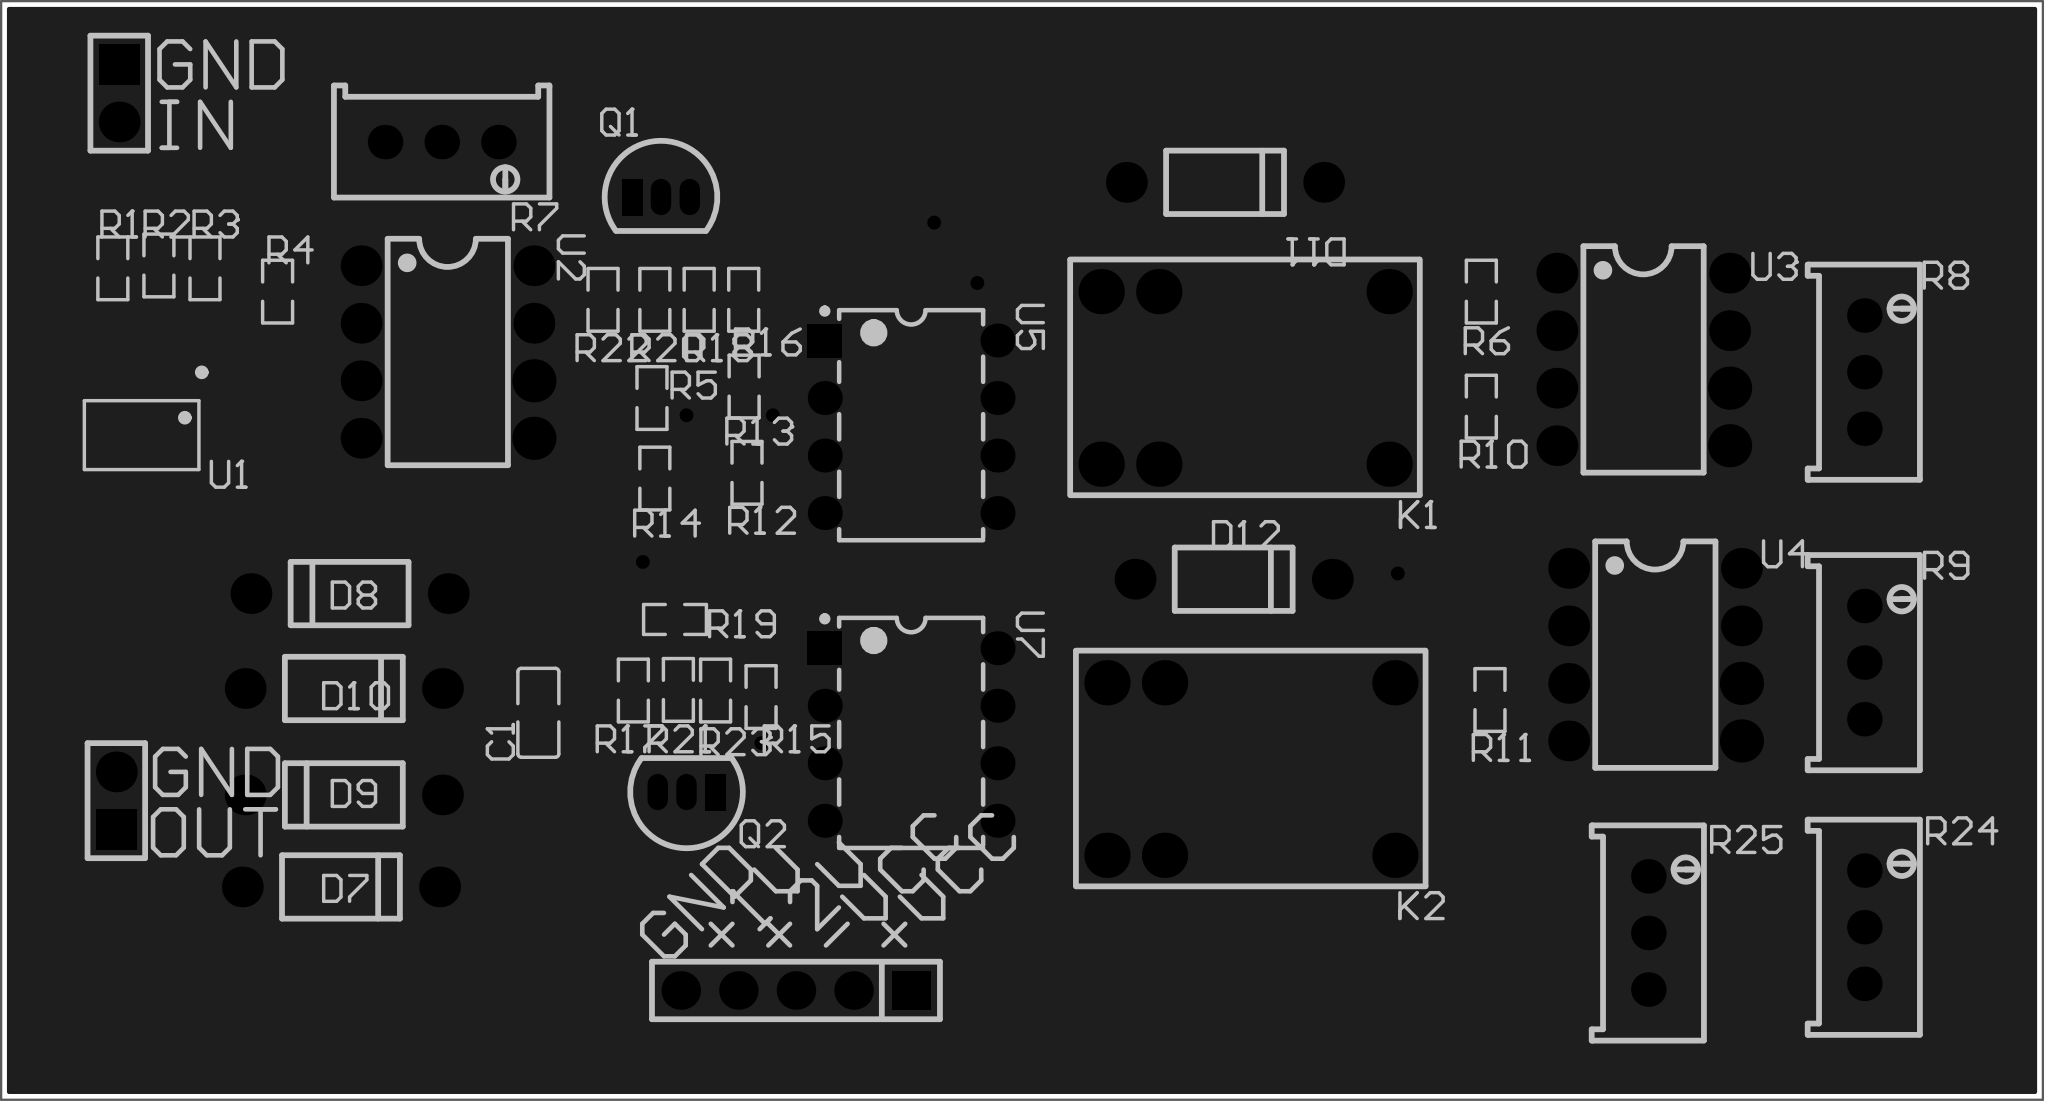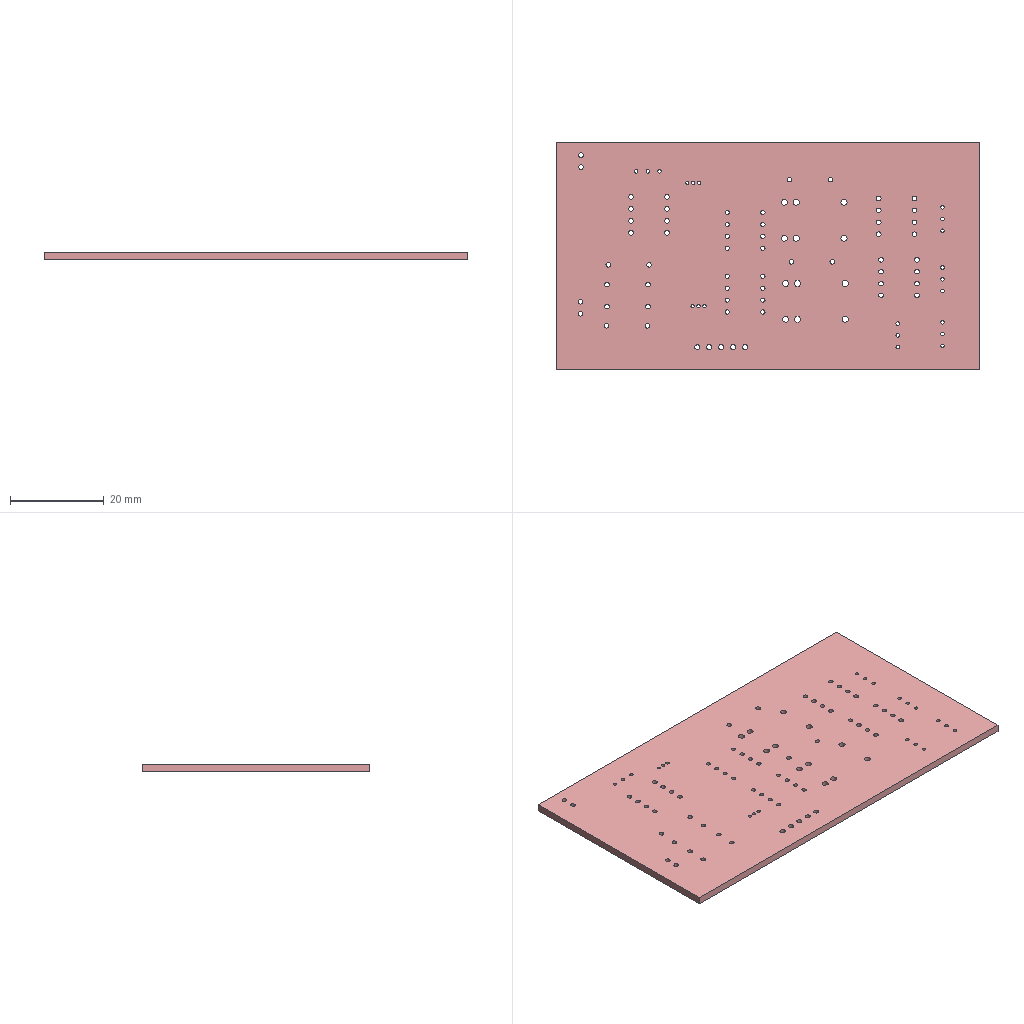Circuit board layout | Altium Designer | box 90 x 48.5 x 1.6 mm
Layer stack:
# Altium Designer layer stack of  (unit mm; dielectric type: 0 none, 1 core, 2 prepreg, 3 surface material)
index,name,kind,layer,copper_thickness_mm,dielectric_type,dielectric_thickness_mm,dielectric_material,dielectric_constant
0,Top Paste Mask Layer,other,,,,,,
1,Top Silkscreen Layer,other,,,,,,
2,Top Solder Mask Layer,dielectric,,,3,0.01,,3.3
3,Top Layer,copper,Top Layer,0.035,,,,
4,Dielectric1,dielectric,,,3,1.51,FR4,4.5
5,Bottom Layer,copper,Bottom Layer,0.035,,,,
6,Bottom Solder Mask Layer,dielectric,,,3,0.01,,3.3
7,Bottom Silkscreen Layer,other,,,,,,
8,Bottom Paste Mask Layer,other,,,,,,
# drill layer pairs: low layer,high layer
drill_pair,Top Layer,Bottom Layer
Part placement:
Designator,Comment,Layer,Footprint,Center-X(mm),Center-Y(mm),Rotation
C1,22uf,TopLayer,C0805,103.575,96.209,90
D7,1N4001-TP,TopLayer,DO-41_BD2.4-L4.7-P8.70-D0.9-RD,94.869,88.519,180
D8,1N4001-TP,TopLayer,DO-41_BD2.4-L4.7-P8.70-D0.9-RD,95.25,101.473,0
D9,1N4001-TP,TopLayer,DO-41_BD2.4-L4.7-P8.70-D0.9-RD,94.996,92.583,0
D10,1N4001-TP,TopLayer,DO-41_BD2.4-L4.7-P8.70-D0.9-RD,94.996,97.282,180
D11,1N4148,TopLayer,DO-41_BD2.4-L4.7-P8.70-D0.9-RD,133.858,119.634,180
D12,1N4148,TopLayer,DO-41_BD2.4-L4.7-P8.70-D0.9-RD,134.239,102.108,180
H1,,TopLayer,HDR-TH_2P-P2.54-V-M-1,85.09,123.571,270
K1,HRS1H-S-DC5V,TopLayer,RELAY-TH_HRS1H-S-DC3V,134.747,110.998,180
K2,HRS1H-S-DC5V,TopLayer,RELAY-TH_HRS1H-S-DC3V,135.001,93.726,180
R7,10kΩ,TopLayer,R_3296,99.314,121.412,180
Q1,2N3904,TopLayer,TO-92-3_L4.9-W3.7-P1.27-L,108.983,118.985,0
Q2,2N3904,TopLayer,TO-92-3_L4.9-W3.7-P1.27-L,110.109,92.71,180
R1,10K,TopLayer,R0603,84.809,115.836,270
R2,10K,TopLayer,R0603,86.841,115.963,270
R3,1K,TopLayer,R0603,88.873,115.836,270
R4,1K,TopLayer,R0603,92.075,114.808,270
R5,1K,TopLayer,R0603,108.585,110.109,270
R6,1K,TopLayer,R0603,145.161,114.808,90
R8,10kΩ,TopLayer,R_3296,162.052,111.252,270
R9,10kΩ,TopLayer,R_3296,162.052,98.425,270
R10,1K,TopLayer,R0603,145.161,109.728,90
R11,1K,TopLayer,R0603,145.542,96.774,90
R12,1K,TopLayer,R0603,112.776,106.807,90
R13,1K,TopLayer,R0603,112.649,110.617,90
R14,1K,TopLayer,R0603,108.712,106.553,270
R15,1K,TopLayer,R0603,113.396,96.904,90
R16,3K,TopLayer,R0603,112.63,114.445,270
R17,3K,TopLayer,R0603,107.764,97.192,90
R18,1K,TopLayer,R0603,110.667,114.445,90
R19,1K,TopLayer,R0603,109.601,100.33,180
R20,1K,TopLayer,R0603,108.712,114.445,90
R21,1K,TopLayer,R0603,109.75,97.219,270
R22,1K,TopLayer,R0603,106.426,114.445,270
R23,1K,TopLayer,R0603,111.391,97.193,90
R25,100kΩ,TopLayer,R_3296,152.527,86.487,270
R24,100kΩ,TopLayer,R_3296,162.052,86.741,270
U1,LF353D,TopLayer,SOIC-8_L4.9-W3.9-P1.27-LS6.0-BL,86.079,108.47,180
U2,ADOP37AQ,TopLayer,PDIP-8_L9.6-W6.4-P2.54-LS7.6-BL,99.568,112.141,270
U3,ADOP37AQ,TopLayer,PDIP-8_L9.6-W6.4-P2.54-LS7.6-BL,152.302,111.814,270
U4,ADOP37AQ,TopLayer,PDIP-8_L9.6-W6.4-P2.54-LS7.6-BL,152.822,98.777,270
U5,LM393P,TopLayer,DIP-8_L10.1-W6.3-P2.54-LS7.6-BL-1,120.015,108.839,270
U7,LM393P,TopLayer,DIP-8_L10.1-W6.3-P2.54-LS7.6-BL-1,120.015,95.25,270
H2,,TopLayer,HDR-TH_5P-P2.54-V-M,114.935,83.947,180
H4,,TopLayer,HDR-TH_2P-P2.54-V-M-1,84.963,92.329,90
Pad and via stacks:
# Altium Designer via and pad stacks of  (unit mm). Each distinct definition once, with the count of objects using it.
# via: kind,start_layer,end_layer,hole_mm,diameter_mm,mode(0 simple;1 top-mid-bottom;2 full stack),diameter_per_layer,count,example_net
# pad: kind,layer,hole_mm,hole_type(0 round;1 square;2 slot),plating,top_size,top_shape(1 round;2 rect;3 octagon;9 rounded rect),mid_size,bottom_size,mode,footprint,size_per_layer,count,example
pad,Top Layer,0,0,plated,1.41x1.35,2,1.41x1.35,1.41x1.35,0,C0805,,2,C1.2
pad,Top Layer,0,0,plated,0.8065x0.864,2,0.8065x0.864,0.8065x0.864,0,R0603,,40,R1.2
pad,Top Layer,0,0,plated,0.588x2.045,1,0.588x2.045,0.588x2.045,0,SOIC-8_L4.9-W3.9-P1.27-LS6.0-BL,,8,U1.1
pad,Multi-Layer,1,0,plated,1.8x1.8,1,1.8x1.8,1.8x1.8,0,DO-41_BD2.4-L4.7-P8.70-D0.9-RD,,12,D7.1
pad,Multi-Layer,1,0,plated,1.8x1.8,1,1.8x1.8,1.8x1.8,0,HDR-TH_2P-P2.54-V-M-1,,2,H1.2
pad,Multi-Layer,1,0,plated,1.8x1.8,2,1.8x1.8,1.8x1.8,0,HDR-TH_2P-P2.54-V-M-1,,2,H1.1
pad,Multi-Layer,1.3,0,plated,2x2,1,2x2,2x2,0,RELAY-TH_HRS1H-S-DC3V,,12,K1.1
pad,Multi-Layer,0.762,0,plated,1.524x1.524,1,1.524x1.524,1.524x1.524,0,R_3296,,15,R7.2
pad,Multi-Layer,0.7,0,plated,0.9x1.6,1,0.9x1.6,0.9x1.6,0,TO-92-3_L4.9-W3.7-P1.27-L,,4,Q1.3
pad,Multi-Layer,0.7,0,plated,0.9x1.6,2,0.9x1.6,0.9x1.6,0,TO-92-3_L4.9-W3.7-P1.27-L,,2,Q1.1
pad,Multi-Layer,1,0,plated,1.8x1.8,1,1.8x1.8,1.8x1.8,0,PDIP-8_L9.6-W6.4-P2.54-LS7.6-BL,,18,U2.1
pad,Multi-Layer,1,0,plated,1.905x1.905,1,1.905x1.905,1.905x1.905,0,PDIP-8_L9.6-W6.4-P2.54-LS7.6-BL,,6,U2.5
pad,Multi-Layer,0.9,0,plated,1.5x1.5,1,1.5x1.5,1.5x1.5,0,DIP-8_L10.1-W6.3-P2.54-LS7.6-BL-1,,14,U5.5
pad,Multi-Layer,0.9,0,plated,1.5x1.5,2,1.5x1.5,1.5x1.5,0,DIP-8_L10.1-W6.3-P2.54-LS7.6-BL-1,,2,U5.1
pad,Multi-Layer,1.1,0,plated,1.7x1.7,2,1.7x1.7,1.7x1.7,0,HDR-TH_5P-P2.54-V-M,,1,H2.1
pad,Multi-Layer,1.1,0,plated,1.7x1.7,1,1.7x1.7,1.7x1.7,0,HDR-TH_5P-P2.54-V-M,,4,H2.2
via,Top Layer,Bottom Layer,0.3048,0.61,0,,5,$1N1453
via,Top Layer,Bottom Layer,0.3048,0.6096,0,,2,1V
Copper pours:
name,layer,net,type(0 solid;1 hatched;2 none)
Top Layer-GND,Top Layer,GND,0
Bottom Layer-GND,Bottom Layer,GND,0